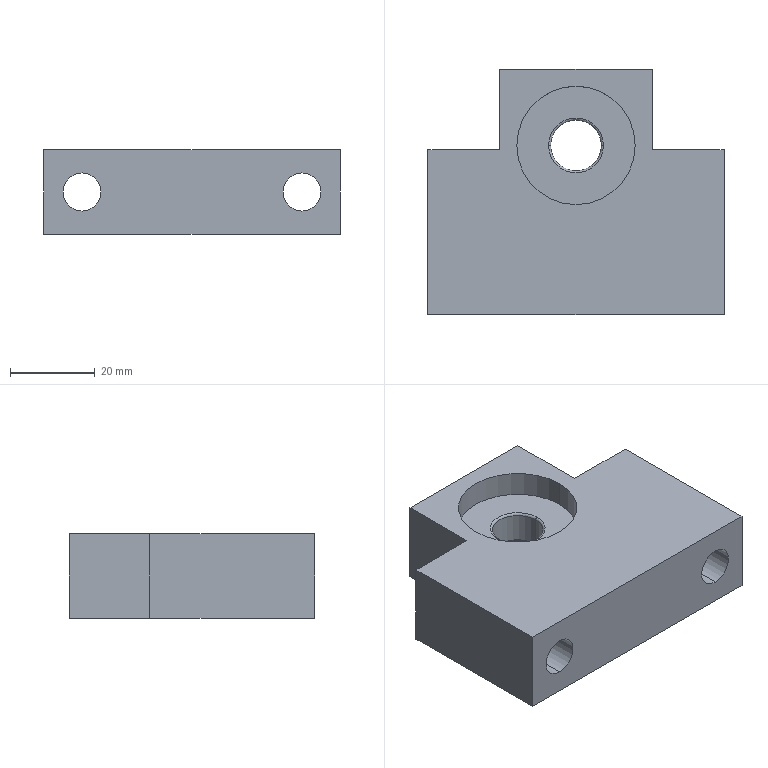Part | STEP file | 0230_006_MTUZ12 | 1 solid | 26 faces | box 70 x 58 x 20 mm | volume 55020 mm3 | plane 12 | cylinder 10 | torus 4 | commonest cylinder face diameters 9 x4 28 x4 12 x2